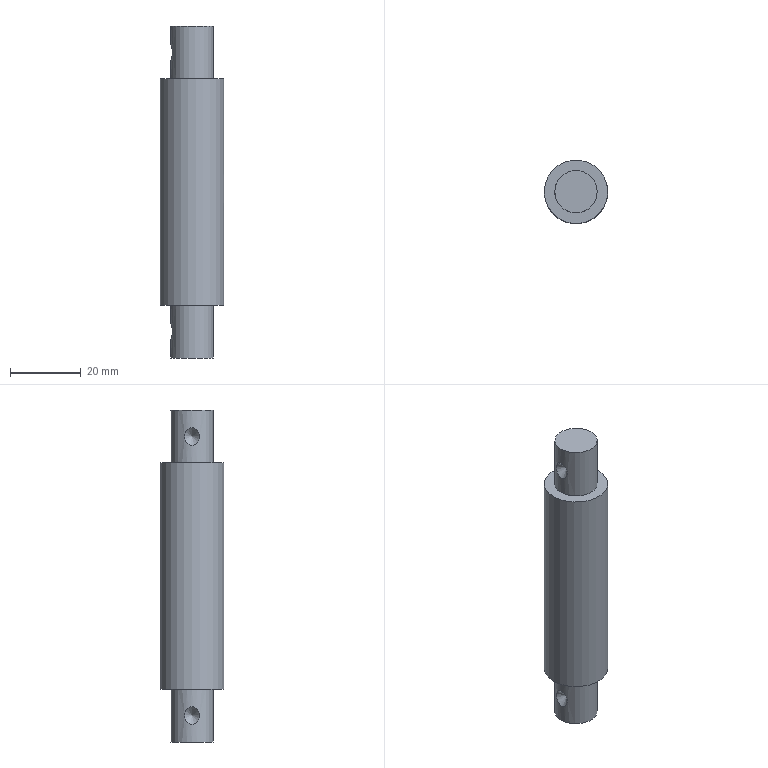Part | NX | features CYLINDER 3, DATUM_CSYS 3, SUBTRACT 3, SKETCH 2, SWP104 2, CHAMFER 1, DATUM_PLANE 1, EXTRUDE 1, SPHERE 1 | 1 solid | 12 faces | box 18 x 18 x 94 mm | volume 19453 mm3 | cylinder 5 | plane 4 | cone 2 | sphere 1 | commonest cylinder face diameters 2 x2 12 x2 18 x1
STEP:
#1=CARTESIAN_POINT('',(9.,0.,15.));
#2=VERTEX_POINT('',#1);
#3=CARTESIAN_POINT('',(0.,0.,15.));
#4=DIRECTION('',(0.,0.,1.));
#5=DIRECTION('',(1.,0.,0.));
#6=AXIS2_PLACEMENT_3D('',#3,#4,#5);
#7=CIRCLE('',#6,9.);
#8=EDGE_CURVE('',#2,#2,#7,.T.);
#9=ORIENTED_EDGE('',*,*,#8,.T.);
#10=EDGE_LOOP('',(#9));
#11=FACE_BOUND('',#10,.T.);
#12=CARTESIAN_POINT('',(9.,0.,79.));
#13=VERTEX_POINT('',#12);
#14=CARTESIAN_POINT('',(0.,0.,79.));
#15=DIRECTION('',(0.,0.,-1.));
#16=DIRECTION('',(1.,0.,0.));
#17=AXIS2_PLACEMENT_3D('',#14,#15,#16);
#18=CIRCLE('',#17,9.);
#19=EDGE_CURVE('',#13,#13,#18,.T.);
#20=ORIENTED_EDGE('',*,*,#19,.T.);
#21=EDGE_LOOP('',(#20));
#22=FACE_BOUND('',#21,.T.);
#23=CARTESIAN_POINT('',(9.,0.,47.));
#24=VERTEX_POINT('',#23);
#25=CARTESIAN_POINT('',(8.972,0.7845,47.217));
#26=CARTESIAN_POINT('',(9.014,-0.0001951,46.892));
#27=CARTESIAN_POINT('',(8.972,-0.7837,47.217));
#28=CARTESIAN_POINT('',(8.93,-1.108,47.999));
#29=CARTESIAN_POINT('',(8.972,-0.784,48.783));
#30=CARTESIAN_POINT('',(9.014,-0.0002087,49.108));
#31=CARTESIAN_POINT('',(8.972,0.7826,48.784));
#32=CARTESIAN_POINT('',(8.93,1.108,48.001));
#33=CARTESIAN_POINT('',(8.972,0.7845,47.217));
#34=CARTESIAN_POINT('',(9.014,-0.0001951,46.892));
#35=CARTESIAN_POINT('',(8.972,-0.7837,47.217));
#36=B_SPLINE_CURVE_WITH_KNOTS('',3,(#25,#26,#27,#28,#29,#30,#31,#32,#33,#34,#35),.UNSPECIFIED.,.T.,.F.,(1,1,1,1,1,1,1,1,1,1,1,1,1,1,1),(-0.002346,-0.001564,-0.0007821,0.,0.0007821,0.001564,0.002346,0.003129,0.003911,0.004693,0.005475,0.006257,0.007039,0.007821,0.008603),.UNSPECIFIED.);
#37=EDGE_CURVE('',#24,#24,#36,.T.);
#38=ORIENTED_EDGE('',*,*,#37,.T.);
#39=EDGE_LOOP('',(#38));
#40=FACE_BOUND('',#39,.T.);
#41=CARTESIAN_POINT('',(0.,0.,15.));
#42=DIRECTION('',(0.,0.,1.));
#43=DIRECTION('',(1.,0.,0.));
#44=AXIS2_PLACEMENT_3D('',#41,#42,#43);
#45=CYLINDRICAL_SURFACE('',#44,9.);
#46=ADVANCED_FACE('',(#11,#22,#40),#45,.T.);
#47=CARTESIAN_POINT('',(-1.,0.,0.));
#48=VERTEX_POINT('',#47);
#49=CARTESIAN_POINT('',(0.,0.,0.));
#50=DIRECTION('',(0.,0.,-1.));
#51=DIRECTION('',(-1.,0.,0.));
#52=AXIS2_PLACEMENT_3D('',#49,#50,#51);
#53=CIRCLE('',#52,1.);
#54=EDGE_CURVE('',#48,#48,#53,.T.);
#55=ORIENTED_EDGE('',*,*,#54,.F.);
#56=EDGE_LOOP('',(#55));
#57=FACE_BOUND('',#56,.T.);
#58=CARTESIAN_POINT('',(6.,0.,0.));
#59=VERTEX_POINT('',#58);
#60=CARTESIAN_POINT('',(0.,0.,0.));
#61=DIRECTION('',(0.,0.,1.));
#62=DIRECTION('',(1.,0.,0.));
#63=AXIS2_PLACEMENT_3D('',#60,#61,#62);
#64=CIRCLE('',#63,6.);
#65=EDGE_CURVE('',#59,#59,#64,.T.);
#66=ORIENTED_EDGE('',*,*,#65,.F.);
#67=EDGE_LOOP('',(#66));
#68=FACE_BOUND('',#67,.T.);
#69=CARTESIAN_POINT('',(0.,0.,0.));
#70=DIRECTION('',(0.,0.,-1.));
#71=DIRECTION('',(-1.,0.,0.));
#72=AXIS2_PLACEMENT_3D('',#69,#70,#71);
#73=PLANE('',#72);
#74=ADVANCED_FACE('',(#57,#68),#73,.T.);
#75=CARTESIAN_POINT('',(-5.874,-1.222,5.464));
#76=VERTEX_POINT('',#75);
#77=CARTESIAN_POINT('',(-6.008,-0.4396,4.972));
#78=CARTESIAN_POINT('',(-5.836,-1.541,5.569));
#79=CARTESIAN_POINT('',(-5.553,-2.262,6.987));
#80=CARTESIAN_POINT('',(-5.676,-2.002,8.874));
#81=CARTESIAN_POINT('',(-5.999,-0.831,9.997));
#82=CARTESIAN_POINT('',(-6.008,0.4411,10.028));
#83=CARTESIAN_POINT('',(-5.837,1.535,9.436));
#84=CARTESIAN_POINT('',(-5.552,2.264,8.014));
#85=CARTESIAN_POINT('',(-5.676,2.002,6.125));
#86=CARTESIAN_POINT('',(-5.999,0.8289,5.003));
#87=CARTESIAN_POINT('',(-6.008,-0.4396,4.972));
#88=CARTESIAN_POINT('',(-5.836,-1.541,5.569));
#89=CARTESIAN_POINT('',(-5.553,-2.262,6.987));
#90=B_SPLINE_CURVE_WITH_KNOTS('',3,(#77,#78,#79,#80,#81,#82,#83,#84,#85,#86,#87,#88,#89),.UNSPECIFIED.,.T.,.F.,(1,1,1,1,1,1,1,1,1,1,1,1,1,1,1,1,1),(-0.003642,-0.001821,-0.0009105,0.,0.001821,0.003642,0.005463,0.006374,0.007284,0.009105,0.01093,0.01275,0.01366,0.01457,0.01639,0.01821,0.02003),.UNSPECIFIED.);
#91=EDGE_CURVE('',#76,#76,#90,.T.);
#92=ORIENTED_EDGE('',*,*,#91,.F.);
#93=EDGE_LOOP('',(#92));
#94=FACE_BOUND('',#93,.T.);
#95=CARTESIAN_POINT('',(6.,0.,15.));
#96=VERTEX_POINT('',#95);
#97=CARTESIAN_POINT('',(0.,0.,15.));
#98=DIRECTION('',(0.,0.,-1.));
#99=DIRECTION('',(1.,0.,0.));
#100=AXIS2_PLACEMENT_3D('',#97,#98,#99);
#101=CIRCLE('',#100,6.);
#102=EDGE_CURVE('',#96,#96,#101,.T.);
#103=ORIENTED_EDGE('',*,*,#102,.T.);
#104=EDGE_LOOP('',(#103));
#105=FACE_BOUND('',#104,.T.);
#106=ORIENTED_EDGE('',*,*,#65,.T.);
#107=EDGE_LOOP('',(#106));
#108=FACE_BOUND('',#107,.T.);
#109=CARTESIAN_POINT('',(0.,0.,0.));
#110=DIRECTION('',(0.,0.,1.));
#111=DIRECTION('',(1.,0.,0.));
#112=AXIS2_PLACEMENT_3D('',#109,#110,#111);
#113=CYLINDRICAL_SURFACE('',#112,6.);
#114=ADVANCED_FACE('',(#94,#105,#108),#113,.T.);
#115=CARTESIAN_POINT('',(6.,0.,79.));
#116=VERTEX_POINT('',#115);
#117=CARTESIAN_POINT('',(0.,0.,79.));
#118=DIRECTION('',(0.,0.,1.));
#119=DIRECTION('',(1.,0.,0.));
#120=AXIS2_PLACEMENT_3D('',#117,#118,#119);
#121=CIRCLE('',#120,6.);
#122=EDGE_CURVE('',#116,#116,#121,.T.);
#123=ORIENTED_EDGE('',*,*,#122,.F.);
#124=EDGE_LOOP('',(#123));
#125=FACE_BOUND('',#124,.T.);
#126=ORIENTED_EDGE('',*,*,#19,.F.);
#127=EDGE_LOOP('',(#126));
#128=FACE_BOUND('',#127,.T.);
#129=CARTESIAN_POINT('',(0.,0.,79.));
#130=DIRECTION('',(0.,0.,1.));
#131=DIRECTION('',(1.,0.,0.));
#132=AXIS2_PLACEMENT_3D('',#129,#130,#131);
#133=PLANE('',#132);
#134=ADVANCED_FACE('',(#125,#128),#133,.T.);
#135=ORIENTED_EDGE('',*,*,#102,.F.);
#136=EDGE_LOOP('',(#135));
#137=FACE_BOUND('',#136,.T.);
#138=ORIENTED_EDGE('',*,*,#8,.F.);
#139=EDGE_LOOP('',(#138));
#140=FACE_BOUND('',#139,.T.);
#141=CARTESIAN_POINT('',(0.,0.,15.));
#142=DIRECTION('',(0.,0.,-1.));
#143=DIRECTION('',(-1.,0.,0.));
#144=AXIS2_PLACEMENT_3D('',#141,#142,#143);
#145=PLANE('',#144);
#146=ADVANCED_FACE('',(#137,#140),#145,.T.);
#147=CARTESIAN_POINT('',(6.,0.,94.));
#148=VERTEX_POINT('',#147);
#149=CARTESIAN_POINT('',(0.,0.,94.));
#150=DIRECTION('',(0.,0.,-1.));
#151=DIRECTION('',(1.,0.,0.));
#152=AXIS2_PLACEMENT_3D('',#149,#150,#151);
#153=CIRCLE('',#152,6.);
#154=EDGE_CURVE('',#148,#148,#153,.T.);
#155=ORIENTED_EDGE('',*,*,#154,.F.);
#156=EDGE_LOOP('',(#155));
#157=FACE_BOUND('',#156,.T.);
#158=CARTESIAN_POINT('',(0.,0.,94.));
#159=DIRECTION('',(0.,0.,1.));
#160=DIRECTION('',(1.,0.,0.));
#161=AXIS2_PLACEMENT_3D('',#158,#159,#160);
#162=PLANE('',#161);
#163=ADVANCED_FACE('',(#157),#162,.T.);
#164=CARTESIAN_POINT('',(-5.874,-1.222,84.464));
#165=VERTEX_POINT('',#164);
#166=CARTESIAN_POINT('',(-6.008,-0.4396,83.972));
#167=CARTESIAN_POINT('',(-5.836,-1.541,84.569));
#168=CARTESIAN_POINT('',(-5.553,-2.262,85.987));
#169=CARTESIAN_POINT('',(-5.676,-2.002,87.874));
#170=CARTESIAN_POINT('',(-5.999,-0.831,88.997));
#171=CARTESIAN_POINT('',(-6.008,0.4411,89.028));
#172=CARTESIAN_POINT('',(-5.837,1.535,88.436));
#173=CARTESIAN_POINT('',(-5.552,2.264,87.014));
#174=CARTESIAN_POINT('',(-5.676,2.002,85.125));
#175=CARTESIAN_POINT('',(-5.999,0.8289,84.003));
#176=CARTESIAN_POINT('',(-6.008,-0.4396,83.972));
#177=CARTESIAN_POINT('',(-5.836,-1.541,84.569));
#178=CARTESIAN_POINT('',(-5.553,-2.262,85.987));
#179=B_SPLINE_CURVE_WITH_KNOTS('',3,(#166,#167,#168,#169,#170,#171,#172,#173,#174,#175,#176,#177,#178),.UNSPECIFIED.,.T.,.F.,(1,1,1,1,1,1,1,1,1,1,1,1,1,1,1,1,1),(-0.003642,-0.001821,-0.0009105,0.,0.001821,0.003642,0.005463,0.006374,0.007284,0.009105,0.01093,0.01275,0.01366,0.01457,0.01639,0.01821,0.02003),.UNSPECIFIED.);
#180=EDGE_CURVE('',#165,#165,#179,.T.);
#181=ORIENTED_EDGE('',*,*,#180,.F.);
#182=EDGE_LOOP('',(#181));
#183=FACE_BOUND('',#182,.T.);
#184=ORIENTED_EDGE('',*,*,#154,.T.);
#185=EDGE_LOOP('',(#184));
#186=FACE_BOUND('',#185,.T.);
#187=ORIENTED_EDGE('',*,*,#122,.T.);
#188=EDGE_LOOP('',(#187));
#189=FACE_BOUND('',#188,.T.);
#190=CARTESIAN_POINT('',(0.,0.,79.));
#191=DIRECTION('',(0.,0.,1.));
#192=DIRECTION('',(1.,0.,0.));
#193=AXIS2_PLACEMENT_3D('',#190,#191,#192);
#194=CYLINDRICAL_SURFACE('',#193,6.);
#195=ADVANCED_FACE('',(#183,#186,#189),#194,.T.);
#196=CARTESIAN_POINT('',(-1.,0.,54.));
#197=VERTEX_POINT('',#196);
#198=CARTESIAN_POINT('',(0.,0.,54.));
#199=DIRECTION('',(0.,0.,-1.));
#200=DIRECTION('',(-1.,0.,0.));
#201=AXIS2_PLACEMENT_3D('',#198,#199,#200);
#202=CIRCLE('',#201,1.);
#203=EDGE_CURVE('',#197,#197,#202,.F.);
#204=ORIENTED_EDGE('',*,*,#203,.T.);
#205=EDGE_LOOP('',(#204));
#206=FACE_BOUND('',#205,.T.);
#207=ORIENTED_EDGE('',*,*,#54,.T.);
#208=EDGE_LOOP('',(#207));
#209=FACE_BOUND('',#208,.T.);
#210=CARTESIAN_POINT('',(0.,1.,48.));
#211=VERTEX_POINT('',#210);
#212=CARTESIAN_POINT('',(0.,-1.,48.));
#213=VERTEX_POINT('',#212);
#214=CARTESIAN_POINT('',(0.,0.,48.));
#215=DIRECTION('',(0.7071,0.,0.7071));
#216=DIRECTION('',(-0.7071,0.,0.7071));
#217=AXIS2_PLACEMENT_3D('',#214,#215,#216);
#218=ELLIPSE('',#217,1.414,1.);
#219=EDGE_CURVE('',#211,#213,#218,.F.);
#220=ORIENTED_EDGE('',*,*,#219,.F.);
#221=CARTESIAN_POINT('',(0.,0.,48.));
#222=DIRECTION('',(-0.7071,0.,0.7071));
#223=DIRECTION('',(0.7071,0.,0.7071));
#224=AXIS2_PLACEMENT_3D('',#221,#222,#223);
#225=ELLIPSE('',#224,1.414,1.);
#226=EDGE_CURVE('',#213,#211,#225,.T.);
#227=ORIENTED_EDGE('',*,*,#226,.F.);
#228=EDGE_LOOP('',(#220,#227));
#229=FACE_BOUND('',#228,.T.);
#230=CARTESIAN_POINT('',(0.,0.,0.));
#231=DIRECTION('',(0.,0.,1.));
#232=DIRECTION('',(1.,0.,0.));
#233=AXIS2_PLACEMENT_3D('',#230,#231,#232);
#234=CYLINDRICAL_SURFACE('',#233,1.);
#235=ADVANCED_FACE('',(#206,#209,#229),#234,.F.);
#236=ORIENTED_EDGE('',*,*,#203,.F.);
#237=EDGE_LOOP('',(#236));
#238=FACE_BOUND('',#237,.T.);
#239=CARTESIAN_POINT('',(0.,0.,54.));
#240=DIRECTION('',(0.,0.,1.));
#241=DIRECTION('',(1.,0.,0.));
#242=AXIS2_PLACEMENT_3D('',#239,#240,#241);
#243=SPHERICAL_SURFACE('',#242,1.);
#244=ADVANCED_FACE('',(#238),#243,.F.);
#245=ORIENTED_EDGE('',*,*,#37,.F.);
#246=EDGE_LOOP('',(#245));
#247=FACE_BOUND('',#246,.T.);
#248=ORIENTED_EDGE('',*,*,#226,.T.);
#249=ORIENTED_EDGE('',*,*,#219,.T.);
#250=EDGE_LOOP('',(#248,#249));
#251=FACE_BOUND('',#250,.T.);
#252=CARTESIAN_POINT('',(0.,0.,48.));
#253=DIRECTION('',(1.,0.,0.));
#254=DIRECTION('',(0.,0.,-1.));
#255=AXIS2_PLACEMENT_3D('',#252,#253,#254);
#256=CYLINDRICAL_SURFACE('',#255,1.);
#257=ADVANCED_FACE('',(#247,#251),#256,.F.);
#258=ORIENTED_EDGE('',*,*,#91,.T.);
#259=EDGE_LOOP('',(#258));
#260=FACE_BOUND('',#259,.T.);
#261=CARTESIAN_POINT('',(-3.5,0.,7.5));
#262=VERTEX_POINT('',#261);
#263=VERTEX_LOOP('',#262);
#264=FACE_BOUND('',#263,.T.);
#265=CARTESIAN_POINT('',(-6.,0.,7.5));
#266=DIRECTION('',(-1.,0.,0.));
#267=DIRECTION('',(0.,0.,1.));
#268=AXIS2_PLACEMENT_3D('',#265,#266,#267);
#269=CONICAL_SURFACE('',#268,2.5,0.7854);
#270=ADVANCED_FACE('',(#260,#264),#269,.F.);
#271=ORIENTED_EDGE('',*,*,#180,.T.);
#272=EDGE_LOOP('',(#271));
#273=FACE_BOUND('',#272,.T.);
#274=CARTESIAN_POINT('',(-3.5,0.,86.5));
#275=VERTEX_POINT('',#274);
#276=VERTEX_LOOP('',#275);
#277=FACE_BOUND('',#276,.T.);
#278=CARTESIAN_POINT('',(-6.,0.,86.5));
#279=DIRECTION('',(-1.,0.,0.));
#280=DIRECTION('',(0.,0.,1.));
#281=AXIS2_PLACEMENT_3D('',#278,#279,#280);
#282=CONICAL_SURFACE('',#281,2.5,0.7854);
#283=ADVANCED_FACE('',(#273,#277),#282,.F.);
#284=CLOSED_SHELL('',(#46,#74,#114,#134,#146,#163,#195,#235,#244,#257,#270,#283));
#285=MANIFOLD_SOLID_BREP('',#284);
#286=(LENGTH_UNIT()NAMED_UNIT(*)SI_UNIT(.MILLI.,.METRE.));
#287=UNCERTAINTY_MEASURE_WITH_UNIT(LENGTH_MEASURE(0.0508),#286,'','');
#288=(NAMED_UNIT(*)PLANE_ANGLE_UNIT()SI_UNIT($,.RADIAN.));
#289=(NAMED_UNIT(*)SI_UNIT($,.STERADIAN.)SOLID_ANGLE_UNIT());
#290=(GEOMETRIC_REPRESENTATION_CONTEXT(3)GLOBAL_UNCERTAINTY_ASSIGNED_CONTEXT((#287))GLOBAL_UNIT_ASSIGNED_CONTEXT((#286,#288,#289))REPRESENTATION_CONTEXT('',''));
#291=ADVANCED_BREP_SHAPE_REPRESENTATION('',(#285),#290);